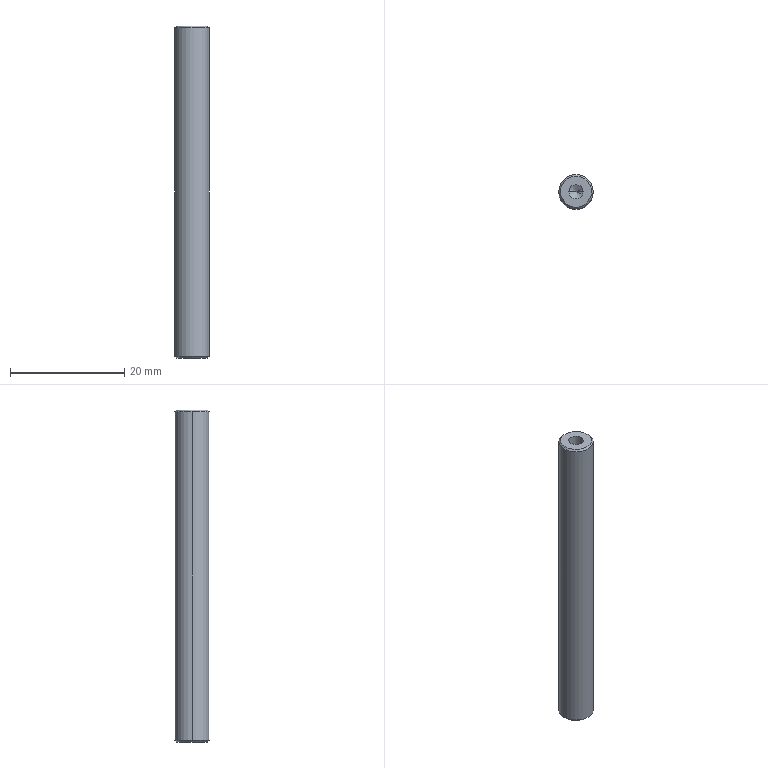Part | STEP file | 10000054268swp000-1 | 1 solid | 16 faces | box 6 x 6 x 58 mm | volume 1518 mm3 | cone 8 | cylinder 6 | plane 2 | commonest cylinder face diameters 2.5 x4 6 x2
STEP:
#1=CARTESIAN_POINT('',(1.25,0.,-17.));
#2=VERTEX_POINT('',#1);
#3=CARTESIAN_POINT('',(-1.25,0.,-17.));
#4=VERTEX_POINT('',#3);
#5=CARTESIAN_POINT('',(0.,0.,-17.));
#6=DIRECTION('',(0.,0.,-1.));
#7=DIRECTION('',(-1.,0.,0.));
#8=AXIS2_PLACEMENT_3D('',#5,#6,#7);
#9=CIRCLE('',#8,1.25);
#10=EDGE_CURVE('',#2,#4,#9,.T.);
#11=ORIENTED_EDGE('',*,*,#10,.F.);
#12=CARTESIAN_POINT('',(1.25,0.,-29.));
#13=VERTEX_POINT('',#12);
#14=CARTESIAN_POINT('',(1.25,0.,-29.));
#15=DIRECTION('',(0.,0.,-1.));
#16=VECTOR('',#15,1000.);
#17=LINE('',#14,#16);
#18=EDGE_CURVE('',#2,#13,#17,.T.);
#19=ORIENTED_EDGE('',*,*,#18,.T.);
#20=CARTESIAN_POINT('',(-1.25,0.,-29.));
#21=VERTEX_POINT('',#20);
#22=CARTESIAN_POINT('',(0.,0.,-29.));
#23=DIRECTION('',(0.,0.,-1.));
#24=DIRECTION('',(-1.,0.,0.));
#25=AXIS2_PLACEMENT_3D('',#22,#23,#24);
#26=CIRCLE('',#25,1.25);
#27=EDGE_CURVE('',#13,#21,#26,.T.);
#28=ORIENTED_EDGE('',*,*,#27,.T.);
#29=CARTESIAN_POINT('',(-1.25,0.,-29.));
#30=DIRECTION('',(0.,0.,-1.));
#31=VECTOR('',#30,1000.);
#32=LINE('',#29,#31);
#33=EDGE_CURVE('',#4,#21,#32,.T.);
#34=ORIENTED_EDGE('',*,*,#33,.F.);
#35=EDGE_LOOP('',(#11,#19,#28,#34));
#36=FACE_OUTER_BOUND('',#35,.T.);
#37=CARTESIAN_POINT('',(0.,0.,-29.));
#38=DIRECTION('',(0.,0.,-1.));
#39=DIRECTION('',(-1.,0.,0.));
#40=AXIS2_PLACEMENT_3D('',#37,#38,#39);
#41=CYLINDRICAL_SURFACE('',#40,1.25);
#42=ADVANCED_FACE('',(#36),#41,.F.);
#43=CARTESIAN_POINT('',(0.,0.,-16.249));
#44=VERTEX_POINT('',#43);
#45=CARTESIAN_POINT('',(-1.25,0.,-17.));
#46=DIRECTION('',(-0.8572,0.,-0.515));
#47=VECTOR('',#46,1000.);
#48=LINE('',#45,#47);
#49=EDGE_CURVE('',#44,#4,#48,.T.);
#50=ORIENTED_EDGE('',*,*,#49,.F.);
#51=CARTESIAN_POINT('',(1.25,0.,-17.));
#52=DIRECTION('',(0.8572,0.,-0.515));
#53=VECTOR('',#52,1000.);
#54=LINE('',#51,#53);
#55=EDGE_CURVE('',#44,#2,#54,.T.);
#56=ORIENTED_EDGE('',*,*,#55,.T.);
#57=ORIENTED_EDGE('',*,*,#10,.T.);
#58=EDGE_LOOP('',(#50,#56,#57));
#59=FACE_OUTER_BOUND('',#58,.T.);
#60=CARTESIAN_POINT('',(0.,0.,-17.));
#61=DIRECTION('',(0.,0.,-1.));
#62=DIRECTION('',(-1.,0.,0.));
#63=AXIS2_PLACEMENT_3D('',#60,#61,#62);
#64=CONICAL_SURFACE('',#63,1.25,1.03);
#65=ADVANCED_FACE('',(#59),#64,.F.);
#66=CARTESIAN_POINT('',(-1.25,0.,17.));
#67=VERTEX_POINT('',#66);
#68=CARTESIAN_POINT('',(1.25,0.,17.));
#69=VERTEX_POINT('',#68);
#70=CARTESIAN_POINT('',(0.,0.,17.));
#71=DIRECTION('',(0.,0.,1.));
#72=DIRECTION('',(1.,0.,0.));
#73=AXIS2_PLACEMENT_3D('',#70,#71,#72);
#74=CIRCLE('',#73,1.25);
#75=EDGE_CURVE('',#67,#69,#74,.T.);
#76=ORIENTED_EDGE('',*,*,#75,.F.);
#77=CARTESIAN_POINT('',(-1.25,0.,29.));
#78=VERTEX_POINT('',#77);
#79=CARTESIAN_POINT('',(-1.25,0.,29.));
#80=DIRECTION('',(0.,0.,1.));
#81=VECTOR('',#80,1000.);
#82=LINE('',#79,#81);
#83=EDGE_CURVE('',#67,#78,#82,.T.);
#84=ORIENTED_EDGE('',*,*,#83,.T.);
#85=CARTESIAN_POINT('',(1.25,0.,29.));
#86=VERTEX_POINT('',#85);
#87=CARTESIAN_POINT('',(0.,0.,29.));
#88=DIRECTION('',(0.,0.,1.));
#89=DIRECTION('',(1.,0.,0.));
#90=AXIS2_PLACEMENT_3D('',#87,#88,#89);
#91=CIRCLE('',#90,1.25);
#92=EDGE_CURVE('',#78,#86,#91,.T.);
#93=ORIENTED_EDGE('',*,*,#92,.T.);
#94=CARTESIAN_POINT('',(1.25,0.,29.));
#95=DIRECTION('',(0.,0.,1.));
#96=VECTOR('',#95,1000.);
#97=LINE('',#94,#96);
#98=EDGE_CURVE('',#69,#86,#97,.T.);
#99=ORIENTED_EDGE('',*,*,#98,.F.);
#100=EDGE_LOOP('',(#76,#84,#93,#99));
#101=FACE_OUTER_BOUND('',#100,.T.);
#102=CARTESIAN_POINT('',(0.,0.,29.));
#103=DIRECTION('',(0.,0.,1.));
#104=DIRECTION('',(1.,0.,0.));
#105=AXIS2_PLACEMENT_3D('',#102,#103,#104);
#106=CYLINDRICAL_SURFACE('',#105,1.25);
#107=ADVANCED_FACE('',(#101),#106,.F.);
#108=CARTESIAN_POINT('',(0.,0.,16.249));
#109=VERTEX_POINT('',#108);
#110=CARTESIAN_POINT('',(1.25,0.,17.));
#111=DIRECTION('',(0.8572,0.,0.515));
#112=VECTOR('',#111,1000.);
#113=LINE('',#110,#112);
#114=EDGE_CURVE('',#109,#69,#113,.T.);
#115=ORIENTED_EDGE('',*,*,#114,.F.);
#116=CARTESIAN_POINT('',(-1.25,0.,17.));
#117=DIRECTION('',(-0.8572,0.,0.515));
#118=VECTOR('',#117,1000.);
#119=LINE('',#116,#118);
#120=EDGE_CURVE('',#109,#67,#119,.T.);
#121=ORIENTED_EDGE('',*,*,#120,.T.);
#122=ORIENTED_EDGE('',*,*,#75,.T.);
#123=EDGE_LOOP('',(#115,#121,#122));
#124=FACE_OUTER_BOUND('',#123,.T.);
#125=CARTESIAN_POINT('',(0.,0.,17.));
#126=DIRECTION('',(0.,0.,1.));
#127=DIRECTION('',(1.,0.,0.));
#128=AXIS2_PLACEMENT_3D('',#125,#126,#127);
#129=CONICAL_SURFACE('',#128,1.25,1.03);
#130=ADVANCED_FACE('',(#124),#129,.F.);
#131=CARTESIAN_POINT('',(2.7,0.,29.));
#132=VERTEX_POINT('',#131);
#133=CARTESIAN_POINT('',(-2.7,0.,29.));
#134=VERTEX_POINT('',#133);
#135=CARTESIAN_POINT('',(0.,0.,29.));
#136=DIRECTION('',(0.,0.,1.));
#137=DIRECTION('',(1.,0.,0.));
#138=AXIS2_PLACEMENT_3D('',#135,#136,#137);
#139=CIRCLE('',#138,2.7);
#140=EDGE_CURVE('',#132,#134,#139,.T.);
#141=ORIENTED_EDGE('',*,*,#140,.F.);
#142=CARTESIAN_POINT('',(3.,0.,28.7));
#143=VERTEX_POINT('',#142);
#144=CARTESIAN_POINT('',(2.7,0.,29.));
#145=DIRECTION('',(0.7071,0.,-0.7071));
#146=VECTOR('',#145,1000.);
#147=LINE('',#144,#146);
#148=EDGE_CURVE('',#132,#143,#147,.T.);
#149=ORIENTED_EDGE('',*,*,#148,.T.);
#150=CARTESIAN_POINT('',(-3.,0.,28.7));
#151=VERTEX_POINT('',#150);
#152=CARTESIAN_POINT('',(0.,0.,28.7));
#153=DIRECTION('',(0.,0.,-1.));
#154=DIRECTION('',(1.,0.,0.));
#155=AXIS2_PLACEMENT_3D('',#152,#153,#154);
#156=CIRCLE('',#155,3.);
#157=EDGE_CURVE('',#151,#143,#156,.T.);
#158=ORIENTED_EDGE('',*,*,#157,.F.);
#159=CARTESIAN_POINT('',(-2.7,0.,29.));
#160=DIRECTION('',(-0.7071,0.,-0.7071));
#161=VECTOR('',#160,1000.);
#162=LINE('',#159,#161);
#163=EDGE_CURVE('',#134,#151,#162,.T.);
#164=ORIENTED_EDGE('',*,*,#163,.F.);
#165=EDGE_LOOP('',(#141,#149,#158,#164));
#166=FACE_OUTER_BOUND('',#165,.T.);
#167=CARTESIAN_POINT('',(0.,0.,29.));
#168=DIRECTION('',(0.,0.,-1.));
#169=DIRECTION('',(-1.,0.,0.));
#170=AXIS2_PLACEMENT_3D('',#167,#168,#169);
#171=CONICAL_SURFACE('',#170,2.7,0.7854);
#172=ADVANCED_FACE('',(#166),#171,.T.);
#173=CARTESIAN_POINT('',(-2.7,0.,-29.));
#174=VERTEX_POINT('',#173);
#175=CARTESIAN_POINT('',(2.7,0.,-29.));
#176=VERTEX_POINT('',#175);
#177=CARTESIAN_POINT('',(0.,0.,-29.));
#178=DIRECTION('',(0.,0.,-1.));
#179=DIRECTION('',(1.,0.,0.));
#180=AXIS2_PLACEMENT_3D('',#177,#178,#179);
#181=CIRCLE('',#180,2.7);
#182=EDGE_CURVE('',#174,#176,#181,.T.);
#183=ORIENTED_EDGE('',*,*,#182,.F.);
#184=CARTESIAN_POINT('',(-3.,0.,-28.7));
#185=VERTEX_POINT('',#184);
#186=CARTESIAN_POINT('',(-3.,0.,-28.7));
#187=DIRECTION('',(-0.7071,0.,0.7071));
#188=VECTOR('',#187,1000.);
#189=LINE('',#186,#188);
#190=EDGE_CURVE('',#174,#185,#189,.T.);
#191=ORIENTED_EDGE('',*,*,#190,.T.);
#192=CARTESIAN_POINT('',(3.,0.,-28.7));
#193=VERTEX_POINT('',#192);
#194=CARTESIAN_POINT('',(0.,0.,-28.7));
#195=DIRECTION('',(0.,0.,1.));
#196=DIRECTION('',(1.,0.,0.));
#197=AXIS2_PLACEMENT_3D('',#194,#195,#196);
#198=CIRCLE('',#197,3.);
#199=EDGE_CURVE('',#193,#185,#198,.T.);
#200=ORIENTED_EDGE('',*,*,#199,.F.);
#201=CARTESIAN_POINT('',(3.,0.,-28.7));
#202=DIRECTION('',(0.7071,0.,0.7071));
#203=VECTOR('',#202,1000.);
#204=LINE('',#201,#203);
#205=EDGE_CURVE('',#176,#193,#204,.T.);
#206=ORIENTED_EDGE('',*,*,#205,.F.);
#207=EDGE_LOOP('',(#183,#191,#200,#206));
#208=FACE_OUTER_BOUND('',#207,.T.);
#209=CARTESIAN_POINT('',(0.,0.,-28.7));
#210=DIRECTION('',(0.,0.,1.));
#211=DIRECTION('',(1.,0.,0.));
#212=AXIS2_PLACEMENT_3D('',#209,#210,#211);
#213=CONICAL_SURFACE('',#212,3.,0.7854);
#214=ADVANCED_FACE('',(#208),#213,.T.);
#215=ORIENTED_EDGE('',*,*,#157,.T.);
#216=CARTESIAN_POINT('',(3.,0.,29.));
#217=DIRECTION('',(0.,0.,-1.));
#218=VECTOR('',#217,1000.);
#219=LINE('',#216,#218);
#220=EDGE_CURVE('',#143,#193,#219,.T.);
#221=ORIENTED_EDGE('',*,*,#220,.T.);
#222=ORIENTED_EDGE('',*,*,#199,.T.);
#223=CARTESIAN_POINT('',(-3.,0.,29.));
#224=DIRECTION('',(0.,0.,-1.));
#225=VECTOR('',#224,1000.);
#226=LINE('',#223,#225);
#227=EDGE_CURVE('',#151,#185,#226,.T.);
#228=ORIENTED_EDGE('',*,*,#227,.F.);
#229=EDGE_LOOP('',(#215,#221,#222,#228));
#230=FACE_OUTER_BOUND('',#229,.T.);
#231=CARTESIAN_POINT('',(0.,0.,29.));
#232=DIRECTION('',(0.,0.,-1.));
#233=DIRECTION('',(-1.,0.,0.));
#234=AXIS2_PLACEMENT_3D('',#231,#232,#233);
#235=CYLINDRICAL_SURFACE('',#234,3.);
#236=ADVANCED_FACE('',(#230),#235,.T.);
#237=ORIENTED_EDGE('',*,*,#220,.F.);
#238=CARTESIAN_POINT('',(0.,0.,28.7));
#239=DIRECTION('',(0.,0.,-1.));
#240=DIRECTION('',(1.,0.,0.));
#241=AXIS2_PLACEMENT_3D('',#238,#239,#240);
#242=CIRCLE('',#241,3.);
#243=EDGE_CURVE('',#143,#151,#242,.T.);
#244=ORIENTED_EDGE('',*,*,#243,.T.);
#245=ORIENTED_EDGE('',*,*,#227,.T.);
#246=CARTESIAN_POINT('',(0.,0.,-28.7));
#247=DIRECTION('',(0.,0.,1.));
#248=DIRECTION('',(1.,0.,0.));
#249=AXIS2_PLACEMENT_3D('',#246,#247,#248);
#250=CIRCLE('',#249,3.);
#251=EDGE_CURVE('',#185,#193,#250,.T.);
#252=ORIENTED_EDGE('',*,*,#251,.T.);
#253=EDGE_LOOP('',(#237,#244,#245,#252));
#254=FACE_OUTER_BOUND('',#253,.T.);
#255=CARTESIAN_POINT('',(0.,0.,29.));
#256=DIRECTION('',(0.,0.,-1.));
#257=DIRECTION('',(-1.,0.,0.));
#258=AXIS2_PLACEMENT_3D('',#255,#256,#257);
#259=CYLINDRICAL_SURFACE('',#258,3.);
#260=ADVANCED_FACE('',(#254),#259,.T.);
#261=CARTESIAN_POINT('',(0.,0.,29.));
#262=DIRECTION('',(0.,0.,1.));
#263=DIRECTION('',(1.,0.,0.));
#264=AXIS2_PLACEMENT_3D('',#261,#262,#263);
#265=CIRCLE('',#264,1.25);
#266=EDGE_CURVE('',#86,#78,#265,.T.);
#267=ORIENTED_EDGE('',*,*,#266,.F.);
#268=ORIENTED_EDGE('',*,*,#92,.F.);
#269=EDGE_LOOP('',(#267,#268));
#270=FACE_BOUND('',#269,.T.);
#271=CARTESIAN_POINT('',(0.,0.,29.));
#272=DIRECTION('',(0.,0.,1.));
#273=DIRECTION('',(1.,0.,0.));
#274=AXIS2_PLACEMENT_3D('',#271,#272,#273);
#275=CIRCLE('',#274,2.7);
#276=EDGE_CURVE('',#134,#132,#275,.T.);
#277=ORIENTED_EDGE('',*,*,#276,.T.);
#278=ORIENTED_EDGE('',*,*,#140,.T.);
#279=EDGE_LOOP('',(#277,#278));
#280=FACE_OUTER_BOUND('',#279,.T.);
#281=CARTESIAN_POINT('',(0.,0.,29.));
#282=DIRECTION('',(0.,0.,1.));
#283=DIRECTION('',(1.,0.,0.));
#284=AXIS2_PLACEMENT_3D('',#281,#282,#283);
#285=PLANE('',#284);
#286=ADVANCED_FACE('',(#270,#280),#285,.T.);
#287=CARTESIAN_POINT('',(0.,0.,-29.));
#288=DIRECTION('',(0.,0.,-1.));
#289=DIRECTION('',(-1.,0.,0.));
#290=AXIS2_PLACEMENT_3D('',#287,#288,#289);
#291=CIRCLE('',#290,1.25);
#292=EDGE_CURVE('',#21,#13,#291,.T.);
#293=ORIENTED_EDGE('',*,*,#292,.F.);
#294=ORIENTED_EDGE('',*,*,#27,.F.);
#295=EDGE_LOOP('',(#293,#294));
#296=FACE_BOUND('',#295,.T.);
#297=CARTESIAN_POINT('',(0.,0.,-29.));
#298=DIRECTION('',(0.,0.,-1.));
#299=DIRECTION('',(1.,0.,0.));
#300=AXIS2_PLACEMENT_3D('',#297,#298,#299);
#301=CIRCLE('',#300,2.7);
#302=EDGE_CURVE('',#176,#174,#301,.T.);
#303=ORIENTED_EDGE('',*,*,#302,.T.);
#304=ORIENTED_EDGE('',*,*,#182,.T.);
#305=EDGE_LOOP('',(#303,#304));
#306=FACE_OUTER_BOUND('',#305,.T.);
#307=CARTESIAN_POINT('',(0.,0.,-29.));
#308=DIRECTION('',(0.,0.,1.));
#309=DIRECTION('',(1.,0.,0.));
#310=AXIS2_PLACEMENT_3D('',#307,#308,#309);
#311=PLANE('',#310);
#312=ADVANCED_FACE('',(#296,#306),#311,.F.);
#313=ORIENTED_EDGE('',*,*,#190,.F.);
#314=ORIENTED_EDGE('',*,*,#302,.F.);
#315=ORIENTED_EDGE('',*,*,#205,.T.);
#316=ORIENTED_EDGE('',*,*,#251,.F.);
#317=EDGE_LOOP('',(#313,#314,#315,#316));
#318=FACE_OUTER_BOUND('',#317,.T.);
#319=CARTESIAN_POINT('',(0.,0.,-28.7));
#320=DIRECTION('',(0.,0.,1.));
#321=DIRECTION('',(1.,0.,0.));
#322=AXIS2_PLACEMENT_3D('',#319,#320,#321);
#323=CONICAL_SURFACE('',#322,3.,0.7854);
#324=ADVANCED_FACE('',(#318),#323,.T.);
#325=ORIENTED_EDGE('',*,*,#148,.F.);
#326=ORIENTED_EDGE('',*,*,#276,.F.);
#327=ORIENTED_EDGE('',*,*,#163,.T.);
#328=ORIENTED_EDGE('',*,*,#243,.F.);
#329=EDGE_LOOP('',(#325,#326,#327,#328));
#330=FACE_OUTER_BOUND('',#329,.T.);
#331=CARTESIAN_POINT('',(0.,0.,29.));
#332=DIRECTION('',(0.,0.,-1.));
#333=DIRECTION('',(-1.,0.,0.));
#334=AXIS2_PLACEMENT_3D('',#331,#332,#333);
#335=CONICAL_SURFACE('',#334,2.7,0.7854);
#336=ADVANCED_FACE('',(#330),#335,.T.);
#337=ORIENTED_EDGE('',*,*,#120,.F.);
#338=ORIENTED_EDGE('',*,*,#114,.T.);
#339=CARTESIAN_POINT('',(0.,0.,17.));
#340=DIRECTION('',(0.,0.,1.));
#341=DIRECTION('',(1.,0.,0.));
#342=AXIS2_PLACEMENT_3D('',#339,#340,#341);
#343=CIRCLE('',#342,1.25);
#344=EDGE_CURVE('',#69,#67,#343,.T.);
#345=ORIENTED_EDGE('',*,*,#344,.T.);
#346=EDGE_LOOP('',(#337,#338,#345));
#347=FACE_OUTER_BOUND('',#346,.T.);
#348=CARTESIAN_POINT('',(0.,0.,17.));
#349=DIRECTION('',(0.,0.,1.));
#350=DIRECTION('',(1.,0.,0.));
#351=AXIS2_PLACEMENT_3D('',#348,#349,#350);
#352=CONICAL_SURFACE('',#351,1.25,1.03);
#353=ADVANCED_FACE('',(#347),#352,.F.);
#354=ORIENTED_EDGE('',*,*,#83,.F.);
#355=ORIENTED_EDGE('',*,*,#344,.F.);
#356=ORIENTED_EDGE('',*,*,#98,.T.);
#357=ORIENTED_EDGE('',*,*,#266,.T.);
#358=EDGE_LOOP('',(#354,#355,#356,#357));
#359=FACE_OUTER_BOUND('',#358,.T.);
#360=CARTESIAN_POINT('',(0.,0.,29.));
#361=DIRECTION('',(0.,0.,1.));
#362=DIRECTION('',(1.,0.,0.));
#363=AXIS2_PLACEMENT_3D('',#360,#361,#362);
#364=CYLINDRICAL_SURFACE('',#363,1.25);
#365=ADVANCED_FACE('',(#359),#364,.F.);
#366=ORIENTED_EDGE('',*,*,#55,.F.);
#367=ORIENTED_EDGE('',*,*,#49,.T.);
#368=CARTESIAN_POINT('',(0.,0.,-17.));
#369=DIRECTION('',(0.,0.,-1.));
#370=DIRECTION('',(-1.,0.,0.));
#371=AXIS2_PLACEMENT_3D('',#368,#369,#370);
#372=CIRCLE('',#371,1.25);
#373=EDGE_CURVE('',#4,#2,#372,.T.);
#374=ORIENTED_EDGE('',*,*,#373,.T.);
#375=EDGE_LOOP('',(#366,#367,#374));
#376=FACE_OUTER_BOUND('',#375,.T.);
#377=CARTESIAN_POINT('',(0.,0.,-17.));
#378=DIRECTION('',(0.,0.,-1.));
#379=DIRECTION('',(-1.,0.,0.));
#380=AXIS2_PLACEMENT_3D('',#377,#378,#379);
#381=CONICAL_SURFACE('',#380,1.25,1.03);
#382=ADVANCED_FACE('',(#376),#381,.F.);
#383=ORIENTED_EDGE('',*,*,#18,.F.);
#384=ORIENTED_EDGE('',*,*,#373,.F.);
#385=ORIENTED_EDGE('',*,*,#33,.T.);
#386=ORIENTED_EDGE('',*,*,#292,.T.);
#387=EDGE_LOOP('',(#383,#384,#385,#386));
#388=FACE_OUTER_BOUND('',#387,.T.);
#389=CARTESIAN_POINT('',(0.,0.,-29.));
#390=DIRECTION('',(0.,0.,-1.));
#391=DIRECTION('',(-1.,0.,0.));
#392=AXIS2_PLACEMENT_3D('',#389,#390,#391);
#393=CYLINDRICAL_SURFACE('',#392,1.25);
#394=ADVANCED_FACE('',(#388),#393,.F.);
#395=CLOSED_SHELL('',(#42,#65,#107,#130,#172,#214,#236,#260,#286,#312,#324,#336,#353,#365,#382,#394));
#396=MANIFOLD_SOLID_BREP('',#395);
#397=CARTESIAN_POINT('',(0.,0.,0.));
#398=DIRECTION('',(0.,0.,1.));
#399=DIRECTION('',(1.,0.,0.));
#400=AXIS2_PLACEMENT_3D('',#397,#398,#399);
#401=(LENGTH_UNIT()NAMED_UNIT(*)SI_UNIT(.MILLI.,.METRE.));
#402=UNCERTAINTY_MEASURE_WITH_UNIT(LENGTH_MEASURE(0.00001),#401,'','');
#403=(NAMED_UNIT(*)PLANE_ANGLE_UNIT()SI_UNIT($,.RADIAN.));
#404=(NAMED_UNIT(*)SI_UNIT($,.STERADIAN.)SOLID_ANGLE_UNIT());
#405=(GEOMETRIC_REPRESENTATION_CONTEXT(3)GLOBAL_UNCERTAINTY_ASSIGNED_CONTEXT((#402))GLOBAL_UNIT_ASSIGNED_CONTEXT((#401,#403,#404))REPRESENTATION_CONTEXT('',''));
#406=ADVANCED_BREP_SHAPE_REPRESENTATION('',(#396,#400),#405);